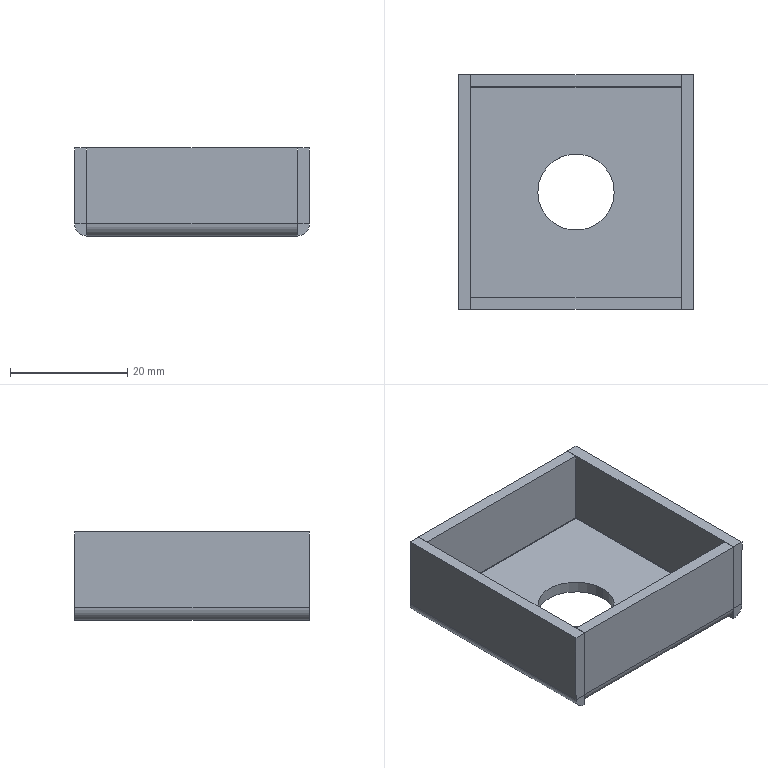Part | SolidWorks | features EdgeFlange 2, FlatPattern 1, ICE 1, SMBaseFlange 1, SheetMetal 1 | 1 solid | 44 faces | box 40 x 40 x 15 mm | volume 6733 mm3 | plane 34 | cylinder 10 | commonest cylinder face diameters 0.2 x4 4.2 x4 13 x2
STEP:
#1=CARTESIAN_POINT('',(-6.5,0.,0.));
#2=VERTEX_POINT('',#1);
#3=CARTESIAN_POINT('',(6.5,0.,0.));
#4=VERTEX_POINT('',#3);
#5=CARTESIAN_POINT('',(0.,0.,0.));
#6=DIRECTION('',(0.,0.,1.));
#7=DIRECTION('',(1.,0.,0.));
#8=AXIS2_PLACEMENT_3D('',#5,#6,#7);
#9=CIRCLE('',#8,6.5);
#10=EDGE_CURVE('',#2,#4,#9,.T.);
#11=ORIENTED_EDGE('',*,*,#10,.T.);
#12=CARTESIAN_POINT('',(6.5,0.,-2.));
#13=VERTEX_POINT('',#12);
#14=CARTESIAN_POINT('',(6.5,0.,8.));
#15=DIRECTION('',(0.,0.,-1.));
#16=VECTOR('',#15,1000.);
#17=LINE('',#14,#16);
#18=EDGE_CURVE('',#4,#13,#17,.T.);
#19=ORIENTED_EDGE('',*,*,#18,.T.);
#20=CARTESIAN_POINT('',(-6.5,0.,-2.));
#21=VERTEX_POINT('',#20);
#22=CARTESIAN_POINT('',(0.,0.,-2.));
#23=DIRECTION('',(0.,0.,-1.));
#24=DIRECTION('',(-1.,0.,0.));
#25=AXIS2_PLACEMENT_3D('',#22,#23,#24);
#26=CIRCLE('',#25,6.5);
#27=EDGE_CURVE('',#13,#21,#26,.T.);
#28=ORIENTED_EDGE('',*,*,#27,.T.);
#29=CARTESIAN_POINT('',(-6.5,0.,8.));
#30=DIRECTION('',(0.,0.,-1.));
#31=VECTOR('',#30,1000.);
#32=LINE('',#29,#31);
#33=EDGE_CURVE('',#2,#21,#32,.T.);
#34=ORIENTED_EDGE('',*,*,#33,.F.);
#35=EDGE_LOOP('',(#11,#19,#28,#34));
#36=FACE_OUTER_BOUND('',#35,.T.);
#37=CARTESIAN_POINT('',(0.,0.,8.));
#38=DIRECTION('',(0.,0.,-1.));
#39=DIRECTION('',(-1.,0.,0.));
#40=AXIS2_PLACEMENT_3D('',#37,#38,#39);
#41=CYLINDRICAL_SURFACE('',#40,6.5);
#42=ADVANCED_FACE('',(#36),#41,.F.);
#43=CARTESIAN_POINT('',(-17.9,-20.,-2.));
#44=VERTEX_POINT('',#43);
#45=CARTESIAN_POINT('',(-17.9,-17.9,-2.));
#46=VERTEX_POINT('',#45);
#47=CARTESIAN_POINT('',(-17.9,-20.,-2.));
#48=DIRECTION('',(0.,1.,0.));
#49=VECTOR('',#48,1000.);
#50=LINE('',#47,#49);
#51=EDGE_CURVE('',#44,#46,#50,.T.);
#52=ORIENTED_EDGE('',*,*,#51,.T.);
#53=CARTESIAN_POINT('',(-17.9,-19.998,0.));
#54=VERTEX_POINT('',#53);
#55=CARTESIAN_POINT('',(-17.9,-17.9,0.1));
#56=DIRECTION('',(-1.,0.,0.));
#57=DIRECTION('',(0.,0.,-1.));
#58=AXIS2_PLACEMENT_3D('',#55,#56,#57);
#59=CIRCLE('',#58,2.1);
#60=EDGE_CURVE('',#46,#54,#59,.T.);
#61=ORIENTED_EDGE('',*,*,#60,.T.);
#62=CARTESIAN_POINT('',(-17.9,-20.,0.));
#63=VERTEX_POINT('',#62);
#64=CARTESIAN_POINT('',(-17.9,-20.,0.));
#65=DIRECTION('',(0.,1.,0.));
#66=VECTOR('',#65,1000.);
#67=LINE('',#64,#66);
#68=EDGE_CURVE('',#63,#54,#67,.T.);
#69=ORIENTED_EDGE('',*,*,#68,.F.);
#70=CARTESIAN_POINT('',(-17.9,-20.,0.));
#71=DIRECTION('',(0.,0.,-1.));
#72=VECTOR('',#71,1000.);
#73=LINE('',#70,#72);
#74=EDGE_CURVE('',#63,#44,#73,.T.);
#75=ORIENTED_EDGE('',*,*,#74,.T.);
#76=EDGE_LOOP('',(#52,#61,#69,#75));
#77=FACE_OUTER_BOUND('',#76,.T.);
#78=CARTESIAN_POINT('',(-17.9,-17.9,0.));
#79=DIRECTION('',(1.,0.,0.));
#80=DIRECTION('',(0.,0.,-1.));
#81=AXIS2_PLACEMENT_3D('',#78,#79,#80);
#82=PLANE('',#81);
#83=ADVANCED_FACE('',(#77),#82,.T.);
#84=CARTESIAN_POINT('',(17.9,-20.,0.));
#85=VERTEX_POINT('',#84);
#86=CARTESIAN_POINT('',(17.9,-19.998,0.));
#87=VERTEX_POINT('',#86);
#88=CARTESIAN_POINT('',(17.9,-20.,0.));
#89=DIRECTION('',(0.,1.,0.));
#90=VECTOR('',#89,1000.);
#91=LINE('',#88,#90);
#92=EDGE_CURVE('',#85,#87,#91,.T.);
#93=ORIENTED_EDGE('',*,*,#92,.T.);
#94=CARTESIAN_POINT('',(17.9,-17.9,-2.));
#95=VERTEX_POINT('',#94);
#96=CARTESIAN_POINT('',(17.9,-17.9,0.1));
#97=DIRECTION('',(1.,0.,0.));
#98=DIRECTION('',(0.,0.,-1.));
#99=AXIS2_PLACEMENT_3D('',#96,#97,#98);
#100=CIRCLE('',#99,2.1);
#101=EDGE_CURVE('',#87,#95,#100,.T.);
#102=ORIENTED_EDGE('',*,*,#101,.T.);
#103=CARTESIAN_POINT('',(17.9,-20.,-2.));
#104=VERTEX_POINT('',#103);
#105=CARTESIAN_POINT('',(17.9,20.,-2.));
#106=DIRECTION('',(0.,1.,0.));
#107=VECTOR('',#106,1000.);
#108=LINE('',#105,#107);
#109=EDGE_CURVE('',#104,#95,#108,.T.);
#110=ORIENTED_EDGE('',*,*,#109,.F.);
#111=CARTESIAN_POINT('',(17.9,-20.,0.));
#112=DIRECTION('',(0.,0.,-1.));
#113=VECTOR('',#112,1000.);
#114=LINE('',#111,#113);
#115=EDGE_CURVE('',#85,#104,#114,.T.);
#116=ORIENTED_EDGE('',*,*,#115,.F.);
#117=EDGE_LOOP('',(#93,#102,#110,#116));
#118=FACE_OUTER_BOUND('',#117,.T.);
#119=CARTESIAN_POINT('',(17.9,-20.,0.));
#120=DIRECTION('',(-1.,0.,0.));
#121=DIRECTION('',(0.,-1.,0.));
#122=AXIS2_PLACEMENT_3D('',#119,#120,#121);
#123=PLANE('',#122);
#124=ADVANCED_FACE('',(#118),#123,.T.);
#125=CARTESIAN_POINT('',(-17.9,20.,0.));
#126=VERTEX_POINT('',#125);
#127=CARTESIAN_POINT('',(-17.9,19.998,0.));
#128=VERTEX_POINT('',#127);
#129=CARTESIAN_POINT('',(-17.9,20.,0.));
#130=DIRECTION('',(0.,-1.,0.));
#131=VECTOR('',#130,1000.);
#132=LINE('',#129,#131);
#133=EDGE_CURVE('',#126,#128,#132,.T.);
#134=ORIENTED_EDGE('',*,*,#133,.T.);
#135=CARTESIAN_POINT('',(-17.9,17.9,-2.));
#136=VERTEX_POINT('',#135);
#137=CARTESIAN_POINT('',(-17.9,17.9,0.1));
#138=DIRECTION('',(-1.,0.,0.));
#139=DIRECTION('',(0.,0.,1.));
#140=AXIS2_PLACEMENT_3D('',#137,#138,#139);
#141=CIRCLE('',#140,2.1);
#142=EDGE_CURVE('',#128,#136,#141,.T.);
#143=ORIENTED_EDGE('',*,*,#142,.T.);
#144=CARTESIAN_POINT('',(-17.9,20.,-2.));
#145=VERTEX_POINT('',#144);
#146=CARTESIAN_POINT('',(-17.9,-20.,-2.));
#147=DIRECTION('',(0.,-1.,0.));
#148=VECTOR('',#147,1000.);
#149=LINE('',#146,#148);
#150=EDGE_CURVE('',#145,#136,#149,.T.);
#151=ORIENTED_EDGE('',*,*,#150,.F.);
#152=CARTESIAN_POINT('',(-17.9,20.,0.));
#153=DIRECTION('',(0.,0.,-1.));
#154=VECTOR('',#153,1000.);
#155=LINE('',#152,#154);
#156=EDGE_CURVE('',#126,#145,#155,.T.);
#157=ORIENTED_EDGE('',*,*,#156,.F.);
#158=EDGE_LOOP('',(#134,#143,#151,#157));
#159=FACE_OUTER_BOUND('',#158,.T.);
#160=CARTESIAN_POINT('',(-17.9,20.,0.));
#161=DIRECTION('',(1.,0.,0.));
#162=DIRECTION('',(0.,0.,-1.));
#163=AXIS2_PLACEMENT_3D('',#160,#161,#162);
#164=PLANE('',#163);
#165=ADVANCED_FACE('',(#159),#164,.T.);
#166=CARTESIAN_POINT('',(17.9,20.,-2.));
#167=VERTEX_POINT('',#166);
#168=CARTESIAN_POINT('',(17.9,17.9,-2.));
#169=VERTEX_POINT('',#168);
#170=CARTESIAN_POINT('',(17.9,20.,-2.));
#171=DIRECTION('',(0.,-1.,0.));
#172=VECTOR('',#171,1000.);
#173=LINE('',#170,#172);
#174=EDGE_CURVE('',#167,#169,#173,.T.);
#175=ORIENTED_EDGE('',*,*,#174,.T.);
#176=CARTESIAN_POINT('',(17.9,19.998,0.));
#177=VERTEX_POINT('',#176);
#178=CARTESIAN_POINT('',(17.9,17.9,0.1));
#179=DIRECTION('',(1.,0.,0.));
#180=DIRECTION('',(0.,0.,1.));
#181=AXIS2_PLACEMENT_3D('',#178,#179,#180);
#182=CIRCLE('',#181,2.1);
#183=EDGE_CURVE('',#169,#177,#182,.T.);
#184=ORIENTED_EDGE('',*,*,#183,.T.);
#185=CARTESIAN_POINT('',(17.9,20.,0.));
#186=VERTEX_POINT('',#185);
#187=CARTESIAN_POINT('',(17.9,20.,0.));
#188=DIRECTION('',(0.,-1.,0.));
#189=VECTOR('',#188,1000.);
#190=LINE('',#187,#189);
#191=EDGE_CURVE('',#186,#177,#190,.T.);
#192=ORIENTED_EDGE('',*,*,#191,.F.);
#193=CARTESIAN_POINT('',(17.9,20.,0.));
#194=DIRECTION('',(0.,0.,-1.));
#195=VECTOR('',#194,1000.);
#196=LINE('',#193,#195);
#197=EDGE_CURVE('',#186,#167,#196,.T.);
#198=ORIENTED_EDGE('',*,*,#197,.T.);
#199=EDGE_LOOP('',(#175,#184,#192,#198));
#200=FACE_OUTER_BOUND('',#199,.T.);
#201=CARTESIAN_POINT('',(17.9,17.9,0.));
#202=DIRECTION('',(-1.,0.,0.));
#203=DIRECTION('',(0.,0.,1.));
#204=AXIS2_PLACEMENT_3D('',#201,#202,#203);
#205=PLANE('',#204);
#206=ADVANCED_FACE('',(#200),#205,.T.);
#207=CARTESIAN_POINT('',(0.,0.,-2.));
#208=DIRECTION('',(0.,0.,-1.));
#209=DIRECTION('',(-1.,0.,0.));
#210=AXIS2_PLACEMENT_3D('',#207,#208,#209);
#211=CIRCLE('',#210,6.5);
#212=EDGE_CURVE('',#21,#13,#211,.T.);
#213=ORIENTED_EDGE('',*,*,#212,.F.);
#214=ORIENTED_EDGE('',*,*,#27,.F.);
#215=EDGE_LOOP('',(#213,#214));
#216=FACE_BOUND('',#215,.T.);
#217=CARTESIAN_POINT('',(17.9,-17.9,-2.));
#218=DIRECTION('',(-1.,0.,0.));
#219=VECTOR('',#218,1000.);
#220=LINE('',#217,#219);
#221=EDGE_CURVE('',#95,#46,#220,.T.);
#222=ORIENTED_EDGE('',*,*,#221,.T.);
#223=CARTESIAN_POINT('',(-17.9,-20.,-2.));
#224=DIRECTION('',(0.,1.,0.));
#225=VECTOR('',#224,1000.);
#226=LINE('',#223,#225);
#227=EDGE_CURVE('',#46,#136,#226,.T.);
#228=ORIENTED_EDGE('',*,*,#227,.T.);
#229=CARTESIAN_POINT('',(-17.9,17.9,-2.));
#230=DIRECTION('',(1.,0.,0.));
#231=VECTOR('',#230,1000.);
#232=LINE('',#229,#231);
#233=EDGE_CURVE('',#136,#169,#232,.T.);
#234=ORIENTED_EDGE('',*,*,#233,.T.);
#235=CARTESIAN_POINT('',(17.9,20.,-2.));
#236=DIRECTION('',(0.,-1.,0.));
#237=VECTOR('',#236,1000.);
#238=LINE('',#235,#237);
#239=EDGE_CURVE('',#169,#95,#238,.T.);
#240=ORIENTED_EDGE('',*,*,#239,.T.);
#241=EDGE_LOOP('',(#222,#228,#234,#240));
#242=FACE_OUTER_BOUND('',#241,.T.);
#243=CARTESIAN_POINT('',(0.,0.,-2.));
#244=DIRECTION('',(0.,0.,1.));
#245=DIRECTION('',(1.,0.,0.));
#246=AXIS2_PLACEMENT_3D('',#243,#244,#245);
#247=PLANE('',#246);
#248=ADVANCED_FACE('',(#216,#242),#247,.F.);
#249=ORIENTED_EDGE('',*,*,#10,.F.);
#250=CARTESIAN_POINT('',(0.,0.,0.));
#251=DIRECTION('',(0.,0.,1.));
#252=DIRECTION('',(1.,0.,0.));
#253=AXIS2_PLACEMENT_3D('',#250,#251,#252);
#254=CIRCLE('',#253,6.5);
#255=EDGE_CURVE('',#4,#2,#254,.T.);
#256=ORIENTED_EDGE('',*,*,#255,.F.);
#257=EDGE_LOOP('',(#249,#256));
#258=FACE_BOUND('',#257,.T.);
#259=CARTESIAN_POINT('',(-17.9,-17.9,0.));
#260=VERTEX_POINT('',#259);
#261=CARTESIAN_POINT('',(-17.9,17.9,0.));
#262=VERTEX_POINT('',#261);
#263=CARTESIAN_POINT('',(-17.9,-20.,0.));
#264=DIRECTION('',(0.,1.,0.));
#265=VECTOR('',#264,1000.);
#266=LINE('',#263,#265);
#267=EDGE_CURVE('',#260,#262,#266,.T.);
#268=ORIENTED_EDGE('',*,*,#267,.F.);
#269=CARTESIAN_POINT('',(17.9,-17.9,0.));
#270=VERTEX_POINT('',#269);
#271=CARTESIAN_POINT('',(17.9,-17.9,0.));
#272=DIRECTION('',(-1.,0.,0.));
#273=VECTOR('',#272,1000.);
#274=LINE('',#271,#273);
#275=EDGE_CURVE('',#270,#260,#274,.T.);
#276=ORIENTED_EDGE('',*,*,#275,.F.);
#277=CARTESIAN_POINT('',(17.9,17.9,0.));
#278=VERTEX_POINT('',#277);
#279=CARTESIAN_POINT('',(17.9,20.,0.));
#280=DIRECTION('',(0.,-1.,0.));
#281=VECTOR('',#280,1000.);
#282=LINE('',#279,#281);
#283=EDGE_CURVE('',#278,#270,#282,.T.);
#284=ORIENTED_EDGE('',*,*,#283,.F.);
#285=CARTESIAN_POINT('',(-17.9,17.9,0.));
#286=DIRECTION('',(1.,0.,0.));
#287=VECTOR('',#286,1000.);
#288=LINE('',#285,#287);
#289=EDGE_CURVE('',#262,#278,#288,.T.);
#290=ORIENTED_EDGE('',*,*,#289,.F.);
#291=EDGE_LOOP('',(#268,#276,#284,#290));
#292=FACE_OUTER_BOUND('',#291,.T.);
#293=CARTESIAN_POINT('',(0.,0.,0.));
#294=DIRECTION('',(0.,0.,1.));
#295=DIRECTION('',(1.,0.,0.));
#296=AXIS2_PLACEMENT_3D('',#293,#294,#295);
#297=PLANE('',#296);
#298=ADVANCED_FACE('',(#258,#292),#297,.T.);
#299=ORIENTED_EDGE('',*,*,#18,.F.);
#300=ORIENTED_EDGE('',*,*,#255,.T.);
#301=ORIENTED_EDGE('',*,*,#33,.T.);
#302=ORIENTED_EDGE('',*,*,#212,.T.);
#303=EDGE_LOOP('',(#299,#300,#301,#302));
#304=FACE_OUTER_BOUND('',#303,.T.);
#305=CARTESIAN_POINT('',(0.,0.,8.));
#306=DIRECTION('',(0.,0.,-1.));
#307=DIRECTION('',(-1.,0.,0.));
#308=AXIS2_PLACEMENT_3D('',#305,#306,#307);
#309=CYLINDRICAL_SURFACE('',#308,6.5);
#310=ADVANCED_FACE('',(#304),#309,.F.);
#311=CARTESIAN_POINT('',(-18.,20.,0.1));
#312=VERTEX_POINT('',#311);
#313=CARTESIAN_POINT('',(-20.,20.,0.1));
#314=VERTEX_POINT('',#313);
#315=CARTESIAN_POINT('',(-20.,20.,0.1));
#316=DIRECTION('',(-1.,0.,0.));
#317=VECTOR('',#316,1000.);
#318=LINE('',#315,#317);
#319=EDGE_CURVE('',#312,#314,#318,.T.);
#320=ORIENTED_EDGE('',*,*,#319,.F.);
#321=CARTESIAN_POINT('',(-17.9,20.,0.1));
#322=DIRECTION('',(0.,1.,0.));
#323=DIRECTION('',(0.,0.,-1.));
#324=AXIS2_PLACEMENT_3D('',#321,#322,#323);
#325=CIRCLE('',#324,0.1);
#326=EDGE_CURVE('',#126,#312,#325,.T.);
#327=ORIENTED_EDGE('',*,*,#326,.F.);
#328=ORIENTED_EDGE('',*,*,#156,.T.);
#329=CARTESIAN_POINT('',(-17.9,20.,0.1));
#330=DIRECTION('',(0.,1.,0.));
#331=DIRECTION('',(0.,0.,-1.));
#332=AXIS2_PLACEMENT_3D('',#329,#330,#331);
#333=CIRCLE('',#332,2.1);
#334=EDGE_CURVE('',#145,#314,#333,.T.);
#335=ORIENTED_EDGE('',*,*,#334,.T.);
#336=EDGE_LOOP('',(#320,#327,#328,#335));
#337=FACE_OUTER_BOUND('',#336,.T.);
#338=CARTESIAN_POINT('',(-17.9,20.,0.1));
#339=DIRECTION('',(0.,1.,0.));
#340=DIRECTION('',(0.,0.,1.));
#341=AXIS2_PLACEMENT_3D('',#338,#339,#340);
#342=PLANE('',#341);
#343=ADVANCED_FACE('',(#337),#342,.T.);
#344=CARTESIAN_POINT('',(-18.,-20.,0.1));
#345=VERTEX_POINT('',#344);
#346=CARTESIAN_POINT('',(-17.9,-20.,0.1));
#347=DIRECTION('',(0.,-1.,0.));
#348=DIRECTION('',(0.,0.,-1.));
#349=AXIS2_PLACEMENT_3D('',#346,#347,#348);
#350=CIRCLE('',#349,0.1);
#351=EDGE_CURVE('',#345,#63,#350,.T.);
#352=ORIENTED_EDGE('',*,*,#351,.F.);
#353=CARTESIAN_POINT('',(-20.,-20.,0.1));
#354=VERTEX_POINT('',#353);
#355=CARTESIAN_POINT('',(-18.,-20.,0.1));
#356=DIRECTION('',(-1.,0.,0.));
#357=VECTOR('',#356,1000.);
#358=LINE('',#355,#357);
#359=EDGE_CURVE('',#345,#354,#358,.T.);
#360=ORIENTED_EDGE('',*,*,#359,.T.);
#361=CARTESIAN_POINT('',(-17.9,-20.,0.1));
#362=DIRECTION('',(0.,-1.,0.));
#363=DIRECTION('',(0.,0.,-1.));
#364=AXIS2_PLACEMENT_3D('',#361,#362,#363);
#365=CIRCLE('',#364,2.1);
#366=EDGE_CURVE('',#354,#44,#365,.T.);
#367=ORIENTED_EDGE('',*,*,#366,.T.);
#368=ORIENTED_EDGE('',*,*,#74,.F.);
#369=EDGE_LOOP('',(#352,#360,#367,#368));
#370=FACE_OUTER_BOUND('',#369,.T.);
#371=CARTESIAN_POINT('',(-17.9,-20.,0.1));
#372=DIRECTION('',(0.,1.,0.));
#373=DIRECTION('',(0.,0.,1.));
#374=AXIS2_PLACEMENT_3D('',#371,#372,#373);
#375=PLANE('',#374);
#376=ADVANCED_FACE('',(#370),#375,.F.);
#377=ORIENTED_EDGE('',*,*,#51,.F.);
#378=ORIENTED_EDGE('',*,*,#366,.F.);
#379=CARTESIAN_POINT('',(-20.,0.,0.1));
#380=DIRECTION('',(0.,-1.,0.));
#381=VECTOR('',#380,1000.);
#382=LINE('',#379,#381);
#383=EDGE_CURVE('',#314,#354,#382,.T.);
#384=ORIENTED_EDGE('',*,*,#383,.F.);
#385=ORIENTED_EDGE('',*,*,#334,.F.);
#386=ORIENTED_EDGE('',*,*,#150,.T.);
#387=ORIENTED_EDGE('',*,*,#227,.F.);
#388=EDGE_LOOP('',(#377,#378,#384,#385,#386,#387));
#389=FACE_OUTER_BOUND('',#388,.T.);
#390=CARTESIAN_POINT('',(-17.9,-20.,0.1));
#391=DIRECTION('',(0.,-1.,0.));
#392=DIRECTION('',(-1.,0.,0.));
#393=AXIS2_PLACEMENT_3D('',#390,#391,#392);
#394=CYLINDRICAL_SURFACE('',#393,2.1);
#395=ADVANCED_FACE('',(#389),#394,.T.);
#396=ORIENTED_EDGE('',*,*,#68,.T.);
#397=CARTESIAN_POINT('',(-17.9,-20.,0.));
#398=DIRECTION('',(0.,1.,0.));
#399=VECTOR('',#398,1000.);
#400=LINE('',#397,#399);
#401=EDGE_CURVE('',#54,#260,#400,.T.);
#402=ORIENTED_EDGE('',*,*,#401,.T.);
#403=ORIENTED_EDGE('',*,*,#267,.T.);
#404=CARTESIAN_POINT('',(-17.9,20.,0.));
#405=DIRECTION('',(0.,-1.,0.));
#406=VECTOR('',#405,1000.);
#407=LINE('',#404,#406);
#408=EDGE_CURVE('',#128,#262,#407,.T.);
#409=ORIENTED_EDGE('',*,*,#408,.F.);
#410=ORIENTED_EDGE('',*,*,#133,.F.);
#411=ORIENTED_EDGE('',*,*,#326,.T.);
#412=CARTESIAN_POINT('',(-18.,20.,0.1));
#413=DIRECTION('',(0.,-1.,0.));
#414=VECTOR('',#413,1000.);
#415=LINE('',#412,#414);
#416=EDGE_CURVE('',#312,#345,#415,.T.);
#417=ORIENTED_EDGE('',*,*,#416,.T.);
#418=ORIENTED_EDGE('',*,*,#351,.T.);
#419=EDGE_LOOP('',(#396,#402,#403,#409,#410,#411,#417,#418));
#420=FACE_OUTER_BOUND('',#419,.T.);
#421=CARTESIAN_POINT('',(-17.9,-20.,0.1));
#422=DIRECTION('',(0.,-1.,0.));
#423=DIRECTION('',(-1.,0.,0.));
#424=AXIS2_PLACEMENT_3D('',#421,#422,#423);
#425=CYLINDRICAL_SURFACE('',#424,0.1);
#426=ADVANCED_FACE('',(#420),#425,.F.);
#427=CARTESIAN_POINT('',(-20.,-20.,13.));
#428=VERTEX_POINT('',#427);
#429=CARTESIAN_POINT('',(-20.,-20.,0.));
#430=DIRECTION('',(0.,0.,-1.));
#431=VECTOR('',#430,1000.);
#432=LINE('',#429,#431);
#433=EDGE_CURVE('',#428,#354,#432,.T.);
#434=ORIENTED_EDGE('',*,*,#433,.T.);
#435=ORIENTED_EDGE('',*,*,#359,.F.);
#436=CARTESIAN_POINT('',(-18.,-20.,13.));
#437=VERTEX_POINT('',#436);
#438=CARTESIAN_POINT('',(-18.,-20.,0.));
#439=DIRECTION('',(0.,0.,-1.));
#440=VECTOR('',#439,1000.);
#441=LINE('',#438,#440);
#442=EDGE_CURVE('',#437,#345,#441,.T.);
#443=ORIENTED_EDGE('',*,*,#442,.F.);
#444=CARTESIAN_POINT('',(-20.,-20.,13.));
#445=DIRECTION('',(1.,0.,0.));
#446=VECTOR('',#445,1000.);
#447=LINE('',#444,#446);
#448=EDGE_CURVE('',#428,#437,#447,.T.);
#449=ORIENTED_EDGE('',*,*,#448,.F.);
#450=EDGE_LOOP('',(#434,#435,#443,#449));
#451=FACE_OUTER_BOUND('',#450,.T.);
#452=CARTESIAN_POINT('',(-20.,-20.,0.));
#453=DIRECTION('',(0.,-1.,0.));
#454=DIRECTION('',(1.,0.,0.));
#455=AXIS2_PLACEMENT_3D('',#452,#453,#454);
#456=PLANE('',#455);
#457=ADVANCED_FACE('',(#451),#456,.T.);
#458=CARTESIAN_POINT('',(-18.,20.,13.));
#459=VERTEX_POINT('',#458);
#460=CARTESIAN_POINT('',(-18.,20.,0.));
#461=DIRECTION('',(0.,0.,1.));
#462=VECTOR('',#461,1000.);
#463=LINE('',#460,#462);
#464=EDGE_CURVE('',#312,#459,#463,.T.);
#465=ORIENTED_EDGE('',*,*,#464,.F.);
#466=ORIENTED_EDGE('',*,*,#319,.T.);
#467=CARTESIAN_POINT('',(-20.,20.,13.));
#468=VERTEX_POINT('',#467);
#469=CARTESIAN_POINT('',(-20.,20.,13.));
#470=DIRECTION('',(0.,0.,1.));
#471=VECTOR('',#470,1000.);
#472=LINE('',#469,#471);
#473=EDGE_CURVE('',#314,#468,#472,.T.);
#474=ORIENTED_EDGE('',*,*,#473,.T.);
#475=CARTESIAN_POINT('',(-20.,20.,13.));
#476=DIRECTION('',(1.,0.,0.));
#477=VECTOR('',#476,1000.);
#478=LINE('',#475,#477);
#479=EDGE_CURVE('',#468,#459,#478,.T.);
#480=ORIENTED_EDGE('',*,*,#479,.T.);
#481=EDGE_LOOP('',(#465,#466,#474,#480));
#482=FACE_OUTER_BOUND('',#481,.T.);
#483=CARTESIAN_POINT('',(-20.,20.,13.));
#484=DIRECTION('',(0.,1.,0.));
#485=DIRECTION('',(-1.,0.,0.));
#486=AXIS2_PLACEMENT_3D('',#483,#484,#485);
#487=PLANE('',#486);
#488=ADVANCED_FACE('',(#482),#487,.T.);
#489=ORIENTED_EDGE('',*,*,#473,.F.);
#490=ORIENTED_EDGE('',*,*,#383,.T.);
#491=ORIENTED_EDGE('',*,*,#433,.F.);
#492=CARTESIAN_POINT('',(-20.,-20.,13.));
#493=DIRECTION('',(0.,-1.,0.));
#494=VECTOR('',#493,1000.);
#495=LINE('',#492,#494);
#496=EDGE_CURVE('',#468,#428,#495,.T.);
#497=ORIENTED_EDGE('',*,*,#496,.F.);
#498=EDGE_LOOP('',(#489,#490,#491,#497));
#499=FACE_OUTER_BOUND('',#498,.T.);
#500=CARTESIAN_POINT('',(-20.,0.,0.));
#501=DIRECTION('',(-1.,0.,0.));
#502=DIRECTION('',(0.,0.,1.));
#503=AXIS2_PLACEMENT_3D('',#500,#501,#502);
#504=PLANE('',#503);
#505=ADVANCED_FACE('',(#499),#504,.T.);
#506=ORIENTED_EDGE('',*,*,#416,.F.);
#507=ORIENTED_EDGE('',*,*,#464,.T.);
#508=CARTESIAN_POINT('',(-18.,0.,13.));
#509=DIRECTION('',(0.,-1.,0.));
#510=VECTOR('',#509,1000.);
#511=LINE('',#508,#510);
#512=EDGE_CURVE('',#459,#437,#511,.T.);
#513=ORIENTED_EDGE('',*,*,#512,.T.);
#514=ORIENTED_EDGE('',*,*,#442,.T.);
#515=EDGE_LOOP('',(#506,#507,#513,#514));
#516=FACE_OUTER_BOUND('',#515,.T.);
#517=CARTESIAN_POINT('',(-18.,0.,0.));
#518=DIRECTION('',(-1.,0.,0.));
#519=DIRECTION('',(0.,0.,1.));
#520=AXIS2_PLACEMENT_3D('',#517,#518,#519);
#521=PLANE('',#520);
#522=ADVANCED_FACE('',(#516),#521,.F.);
#523=ORIENTED_EDGE('',*,*,#512,.F.);
#524=ORIENTED_EDGE('',*,*,#479,.F.);
#525=ORIENTED_EDGE('',*,*,#496,.T.);
#526=ORIENTED_EDGE('',*,*,#448,.T.);
#527=EDGE_LOOP('',(#523,#524,#525,#526));
#528=FACE_OUTER_BOUND('',#527,.T.);
#529=CARTESIAN_POINT('',(-20.,-20.,13.));
#530=DIRECTION('',(0.,0.,1.));
#531=DIRECTION('',(1.,0.,0.));
#532=AXIS2_PLACEMENT_3D('',#529,#530,#531);
#533=PLANE('',#532);
#534=ADVANCED_FACE('',(#528),#533,.T.);
#535=CARTESIAN_POINT('',(18.,-20.,0.1));
#536=VERTEX_POINT('',#535);
#537=CARTESIAN_POINT('',(20.,-20.,0.1));
#538=VERTEX_POINT('',#537);
#539=CARTESIAN_POINT('',(20.,-20.,0.1));
#540=DIRECTION('',(1.,0.,0.));
#541=VECTOR('',#540,1000.);
#542=LINE('',#539,#541);
#543=EDGE_CURVE('',#536,#538,#542,.T.);
#544=ORIENTED_EDGE('',*,*,#543,.F.);
#545=CARTESIAN_POINT('',(17.9,-20.,0.1));
#546=DIRECTION('',(0.,-1.,0.));
#547=DIRECTION('',(0.,0.,1.));
#548=AXIS2_PLACEMENT_3D('',#545,#546,#547);
#549=CIRCLE('',#548,0.1);
#550=EDGE_CURVE('',#85,#536,#549,.T.);
#551=ORIENTED_EDGE('',*,*,#550,.F.);
#552=ORIENTED_EDGE('',*,*,#115,.T.);
#553=CARTESIAN_POINT('',(17.9,-20.,0.1));
#554=DIRECTION('',(0.,-1.,0.));
#555=DIRECTION('',(0.,0.,1.));
#556=AXIS2_PLACEMENT_3D('',#553,#554,#555);
#557=CIRCLE('',#556,2.1);
#558=EDGE_CURVE('',#104,#538,#557,.T.);
#559=ORIENTED_EDGE('',*,*,#558,.T.);
#560=EDGE_LOOP('',(#544,#551,#552,#559));
#561=FACE_OUTER_BOUND('',#560,.T.);
#562=CARTESIAN_POINT('',(17.9,-20.,0.1));
#563=DIRECTION('',(0.,-1.,0.));
#564=DIRECTION('',(0.,0.,-1.));
#565=AXIS2_PLACEMENT_3D('',#562,#563,#564);
#566=PLANE('',#565);
#567=ADVANCED_FACE('',(#561),#566,.T.);
#568=CARTESIAN_POINT('',(18.,20.,0.1));
#569=VERTEX_POINT('',#568);
#570=CARTESIAN_POINT('',(17.9,20.,0.1));
#571=DIRECTION('',(0.,1.,0.));
#572=DIRECTION('',(0.,0.,1.));
#573=AXIS2_PLACEMENT_3D('',#570,#571,#572);
#574=CIRCLE('',#573,0.1);
#575=EDGE_CURVE('',#569,#186,#574,.T.);
#576=ORIENTED_EDGE('',*,*,#575,.F.);
#577=CARTESIAN_POINT('',(20.,20.,0.1));
#578=VERTEX_POINT('',#577);
#579=CARTESIAN_POINT('',(18.,20.,0.1));
#580=DIRECTION('',(1.,0.,0.));
#581=VECTOR('',#580,1000.);
#582=LINE('',#579,#581);
#583=EDGE_CURVE('',#569,#578,#582,.T.);
#584=ORIENTED_EDGE('',*,*,#583,.T.);
#585=CARTESIAN_POINT('',(17.9,20.,0.1));
#586=DIRECTION('',(0.,1.,0.));
#587=DIRECTION('',(0.,0.,1.));
#588=AXIS2_PLACEMENT_3D('',#585,#586,#587);
#589=CIRCLE('',#588,2.1);
#590=EDGE_CURVE('',#578,#167,#589,.T.);
#591=ORIENTED_EDGE('',*,*,#590,.T.);
#592=ORIENTED_EDGE('',*,*,#197,.F.);
#593=EDGE_LOOP('',(#576,#584,#591,#592));
#594=FACE_OUTER_BOUND('',#593,.T.);
#595=CARTESIAN_POINT('',(17.9,20.,0.1));
#596=DIRECTION('',(0.,-1.,0.));
#597=DIRECTION('',(0.,0.,-1.));
#598=AXIS2_PLACEMENT_3D('',#595,#596,#597);
#599=PLANE('',#598);
#600=ADVANCED_FACE('',(#594),#599,.F.);
#601=ORIENTED_EDGE('',*,*,#174,.F.);
#602=ORIENTED_EDGE('',*,*,#590,.F.);
#603=CARTESIAN_POINT('',(20.,-20.,0.1));
#604=DIRECTION('',(0.,-1.,0.));
#605=VECTOR('',#604,1000.);
#606=LINE('',#603,#605);
#607=EDGE_CURVE('',#578,#538,#606,.T.);
#608=ORIENTED_EDGE('',*,*,#607,.T.);
#609=ORIENTED_EDGE('',*,*,#558,.F.);
#610=ORIENTED_EDGE('',*,*,#109,.T.);
#611=ORIENTED_EDGE('',*,*,#239,.F.);
#612=EDGE_LOOP('',(#601,#602,#608,#609,#610,#611));
#613=FACE_OUTER_BOUND('',#612,.T.);
#614=CARTESIAN_POINT('',(17.9,20.,0.1));
#615=DIRECTION('',(0.,1.,0.));
#616=DIRECTION('',(1.,0.,0.));
#617=AXIS2_PLACEMENT_3D('',#614,#615,#616);
#618=CYLINDRICAL_SURFACE('',#617,2.1);
#619=ADVANCED_FACE('',(#613),#618,.T.);
#620=ORIENTED_EDGE('',*,*,#191,.T.);
#621=CARTESIAN_POINT('',(17.9,20.,0.));
#622=DIRECTION('',(0.,-1.,0.));
#623=VECTOR('',#622,1000.);
#624=LINE('',#621,#623);
#625=EDGE_CURVE('',#177,#278,#624,.T.);
#626=ORIENTED_EDGE('',*,*,#625,.T.);
#627=ORIENTED_EDGE('',*,*,#283,.T.);
#628=CARTESIAN_POINT('',(17.9,-20.,0.));
#629=DIRECTION('',(0.,1.,0.));
#630=VECTOR('',#629,1000.);
#631=LINE('',#628,#630);
#632=EDGE_CURVE('',#87,#270,#631,.T.);
#633=ORIENTED_EDGE('',*,*,#632,.F.);
#634=ORIENTED_EDGE('',*,*,#92,.F.);
#635=ORIENTED_EDGE('',*,*,#550,.T.);
#636=CARTESIAN_POINT('',(18.,-20.,0.1));
#637=DIRECTION('',(0.,1.,0.));
#638=VECTOR('',#637,1000.);
#639=LINE('',#636,#638);
#640=EDGE_CURVE('',#536,#569,#639,.T.);
#641=ORIENTED_EDGE('',*,*,#640,.T.);
#642=ORIENTED_EDGE('',*,*,#575,.T.);
#643=EDGE_LOOP('',(#620,#626,#627,#633,#634,#635,#641,#642));
#644=FACE_OUTER_BOUND('',#643,.T.);
#645=CARTESIAN_POINT('',(17.9,20.,0.1));
#646=DIRECTION('',(0.,1.,0.));
#647=DIRECTION('',(1.,0.,0.));
#648=AXIS2_PLACEMENT_3D('',#645,#646,#647);
#649=CYLINDRICAL_SURFACE('',#648,0.1);
#650=ADVANCED_FACE('',(#644),#649,.F.);
#651=CARTESIAN_POINT('',(18.,-20.,13.));
#652=VERTEX_POINT('',#651);
#653=CARTESIAN_POINT('',(18.,-20.,0.));
#654=DIRECTION('',(0.,0.,1.));
#655=VECTOR('',#654,1000.);
#656=LINE('',#653,#655);
#657=EDGE_CURVE('',#536,#652,#656,.T.);
#658=ORIENTED_EDGE('',*,*,#657,.F.);
#659=ORIENTED_EDGE('',*,*,#543,.T.);
#660=CARTESIAN_POINT('',(20.,-20.,13.));
#661=VERTEX_POINT('',#660);
#662=CARTESIAN_POINT('',(20.,-20.,0.));
#663=DIRECTION('',(0.,0.,1.));
#664=VECTOR('',#663,1000.);
#665=LINE('',#662,#664);
#666=EDGE_CURVE('',#538,#661,#665,.T.);
#667=ORIENTED_EDGE('',*,*,#666,.T.);
#668=CARTESIAN_POINT('',(20.,-20.,13.));
#669=DIRECTION('',(-1.,0.,0.));
#670=VECTOR('',#669,1000.);
#671=LINE('',#668,#670);
#672=EDGE_CURVE('',#661,#652,#671,.T.);
#673=ORIENTED_EDGE('',*,*,#672,.T.);
#674=EDGE_LOOP('',(#658,#659,#667,#673));
#675=FACE_OUTER_BOUND('',#674,.T.);
#676=CARTESIAN_POINT('',(20.,-20.,0.));
#677=DIRECTION('',(0.,-1.,0.));
#678=DIRECTION('',(0.,0.,-1.));
#679=AXIS2_PLACEMENT_3D('',#676,#677,#678);
#680=PLANE('',#679);
#681=ADVANCED_FACE('',(#675),#680,.T.);
#682=CARTESIAN_POINT('',(20.,20.,13.));
#683=VERTEX_POINT('',#682);
#684=CARTESIAN_POINT('',(20.,20.,13.));
#685=DIRECTION('',(0.,0.,-1.));
#686=VECTOR('',#685,1000.);
#687=LINE('',#684,#686);
#688=EDGE_CURVE('',#683,#578,#687,.T.);
#689=ORIENTED_EDGE('',*,*,#688,.T.);
#690=ORIENTED_EDGE('',*,*,#583,.F.);
#691=CARTESIAN_POINT('',(18.,20.,13.));
#692=VERTEX_POINT('',#691);
#693=CARTESIAN_POINT('',(18.,20.,0.));
#694=DIRECTION('',(0.,0.,-1.));
#695=VECTOR('',#694,1000.);
#696=LINE('',#693,#695);
#697=EDGE_CURVE('',#692,#569,#696,.T.);
#698=ORIENTED_EDGE('',*,*,#697,.F.);
#699=CARTESIAN_POINT('',(20.,20.,13.));
#700=DIRECTION('',(-1.,0.,0.));
#701=VECTOR('',#700,1000.);
#702=LINE('',#699,#701);
#703=EDGE_CURVE('',#683,#692,#702,.T.);
#704=ORIENTED_EDGE('',*,*,#703,.F.);
#705=EDGE_LOOP('',(#689,#690,#698,#704));
#706=FACE_OUTER_BOUND('',#705,.T.);
#707=CARTESIAN_POINT('',(20.,20.,13.));
#708=DIRECTION('',(0.,1.,0.));
#709=DIRECTION('',(0.,0.,1.));
#710=AXIS2_PLACEMENT_3D('',#707,#708,#709);
#711=PLANE('',#710);
#712=ADVANCED_FACE('',(#706),#711,.T.);
#713=ORIENTED_EDGE('',*,*,#607,.F.);
#714=ORIENTED_EDGE('',*,*,#688,.F.);
#715=CARTESIAN_POINT('',(20.,-20.,13.));
#716=DIRECTION('',(0.,1.,0.));
#717=VECTOR('',#716,1000.);
#718=LINE('',#715,#717);
#719=EDGE_CURVE('',#661,#683,#718,.T.);
#720=ORIENTED_EDGE('',*,*,#719,.F.);
#721=ORIENTED_EDGE('',*,*,#666,.F.);
#722=EDGE_LOOP('',(#713,#714,#720,#721));
#723=FACE_OUTER_BOUND('',#722,.T.);
#724=CARTESIAN_POINT('',(20.,0.,0.));
#725=DIRECTION('',(-1.,0.,0.));
#726=DIRECTION('',(0.,0.,1.));
#727=AXIS2_PLACEMENT_3D('',#724,#725,#726);
#728=PLANE('',#727);
#729=ADVANCED_FACE('',(#723),#728,.F.);
#730=ORIENTED_EDGE('',*,*,#697,.T.);
#731=ORIENTED_EDGE('',*,*,#640,.F.);
#732=ORIENTED_EDGE('',*,*,#657,.T.);
#733=CARTESIAN_POINT('',(18.,0.,13.));
#734=DIRECTION('',(0.,1.,0.));
#735=VECTOR('',#734,1000.);
#736=LINE('',#733,#735);
#737=EDGE_CURVE('',#652,#692,#736,.T.);
#738=ORIENTED_EDGE('',*,*,#737,.T.);
#739=EDGE_LOOP('',(#730,#731,#732,#738));
#740=FACE_OUTER_BOUND('',#739,.T.);
#741=CARTESIAN_POINT('',(18.,0.,0.));
#742=DIRECTION('',(-1.,0.,0.));
#743=DIRECTION('',(0.,0.,1.));
#744=AXIS2_PLACEMENT_3D('',#741,#742,#743);
#745=PLANE('',#744);
#746=ADVANCED_FACE('',(#740),#745,.T.);
#747=ORIENTED_EDGE('',*,*,#737,.F.);
#748=ORIENTED_EDGE('',*,*,#672,.F.);
#749=ORIENTED_EDGE('',*,*,#719,.T.);
#750=ORIENTED_EDGE('',*,*,#703,.T.);
#751=EDGE_LOOP('',(#747,#748,#749,#750));
#752=FACE_OUTER_BOUND('',#751,.T.);
#753=CARTESIAN_POINT('',(20.,-20.,13.));
#754=DIRECTION('',(0.,0.,1.));
#755=DIRECTION('',(1.,0.,0.));
#756=AXIS2_PLACEMENT_3D('',#753,#754,#755);
#757=PLANE('',#756);
#758=ADVANCED_FACE('',(#752),#757,.T.);
#759=ORIENTED_EDGE('',*,*,#625,.F.);
#760=CARTESIAN_POINT('',(17.9,20.,0.1));
#761=VERTEX_POINT('',#760);
#762=CARTESIAN_POINT('',(17.9,17.9,0.1));
#763=DIRECTION('',(1.,0.,0.));
#764=DIRECTION('',(0.,0.,1.));
#765=AXIS2_PLACEMENT_3D('',#762,#763,#764);
#766=CIRCLE('',#765,2.1);
#767=EDGE_CURVE('',#177,#761,#766,.T.);
#768=ORIENTED_EDGE('',*,*,#767,.T.);
#769=CARTESIAN_POINT('',(17.9,18.,0.1));
#770=VERTEX_POINT('',#769);
#771=CARTESIAN_POINT('',(17.9,20.,0.1));
#772=DIRECTION('',(0.,1.,0.));
#773=VECTOR('',#772,1000.);
#774=LINE('',#771,#773);
#775=EDGE_CURVE('',#770,#761,#774,.T.);
#776=ORIENTED_EDGE('',*,*,#775,.F.);
#777=CARTESIAN_POINT('',(17.9,17.9,0.1));
#778=DIRECTION('',(1.,0.,0.));
#779=DIRECTION('',(0.,0.,1.));
#780=AXIS2_PLACEMENT_3D('',#777,#778,#779);
#781=CIRCLE('',#780,0.1);
#782=EDGE_CURVE('',#278,#770,#781,.T.);
#783=ORIENTED_EDGE('',*,*,#782,.F.);
#784=EDGE_LOOP('',(#759,#768,#776,#783));
#785=FACE_OUTER_BOUND('',#784,.T.);
#786=CARTESIAN_POINT('',(17.9,17.9,0.1));
#787=DIRECTION('',(1.,0.,0.));
#788=DIRECTION('',(0.,0.,-1.));
#789=AXIS2_PLACEMENT_3D('',#786,#787,#788);
#790=PLANE('',#789);
#791=ADVANCED_FACE('',(#785),#790,.T.);
#792=CARTESIAN_POINT('',(-17.9,20.,0.1));
#793=VERTEX_POINT('',#792);
#794=CARTESIAN_POINT('',(-17.9,17.9,0.1));
#795=DIRECTION('',(-1.,0.,0.));
#796=DIRECTION('',(0.,0.,1.));
#797=AXIS2_PLACEMENT_3D('',#794,#795,#796);
#798=CIRCLE('',#797,2.1);
#799=EDGE_CURVE('',#793,#128,#798,.T.);
#800=ORIENTED_EDGE('',*,*,#799,.T.);
#801=ORIENTED_EDGE('',*,*,#408,.T.);
#802=CARTESIAN_POINT('',(-17.9,18.,0.1));
#803=VERTEX_POINT('',#802);
#804=CARTESIAN_POINT('',(-17.9,17.9,0.1));
#805=DIRECTION('',(-1.,0.,0.));
#806=DIRECTION('',(0.,0.,1.));
#807=AXIS2_PLACEMENT_3D('',#804,#805,#806);
#808=CIRCLE('',#807,0.1);
#809=EDGE_CURVE('',#803,#262,#808,.T.);
#810=ORIENTED_EDGE('',*,*,#809,.F.);
#811=CARTESIAN_POINT('',(-17.9,18.,0.1));
#812=DIRECTION('',(0.,1.,0.));
#813=VECTOR('',#812,1000.);
#814=LINE('',#811,#813);
#815=EDGE_CURVE('',#803,#793,#814,.T.);
#816=ORIENTED_EDGE('',*,*,#815,.T.);
#817=EDGE_LOOP('',(#800,#801,#810,#816));
#818=FACE_OUTER_BOUND('',#817,.T.);
#819=CARTESIAN_POINT('',(-17.9,17.9,0.1));
#820=DIRECTION('',(1.,0.,0.));
#821=DIRECTION('',(0.,0.,-1.));
#822=AXIS2_PLACEMENT_3D('',#819,#820,#821);
#823=PLANE('',#822);
#824=ADVANCED_FACE('',(#818),#823,.F.);
#825=ORIENTED_EDGE('',*,*,#233,.F.);
#826=ORIENTED_EDGE('',*,*,#142,.F.);
#827=ORIENTED_EDGE('',*,*,#799,.F.);
#828=CARTESIAN_POINT('',(0.,20.,0.1));
#829=DIRECTION('',(-1.,0.,0.));
#830=VECTOR('',#829,1000.);
#831=LINE('',#828,#830);
#832=EDGE_CURVE('',#761,#793,#831,.T.);
#833=ORIENTED_EDGE('',*,*,#832,.F.);
#834=ORIENTED_EDGE('',*,*,#767,.F.);
#835=ORIENTED_EDGE('',*,*,#183,.F.);
#836=EDGE_LOOP('',(#825,#826,#827,#833,#834,#835));
#837=FACE_OUTER_BOUND('',#836,.T.);
#838=CARTESIAN_POINT('',(-17.9,17.9,0.1));
#839=DIRECTION('',(-1.,0.,0.));
#840=DIRECTION('',(0.,1.,0.));
#841=AXIS2_PLACEMENT_3D('',#838,#839,#840);
#842=CYLINDRICAL_SURFACE('',#841,2.1);
#843=ADVANCED_FACE('',(#837),#842,.T.);
#844=ORIENTED_EDGE('',*,*,#289,.T.);
#845=ORIENTED_EDGE('',*,*,#782,.T.);
#846=CARTESIAN_POINT('',(17.9,18.,0.1));
#847=DIRECTION('',(-1.,0.,0.));
#848=VECTOR('',#847,1000.);
#849=LINE('',#846,#848);
#850=EDGE_CURVE('',#770,#803,#849,.T.);
#851=ORIENTED_EDGE('',*,*,#850,.T.);
#852=ORIENTED_EDGE('',*,*,#809,.T.);
#853=EDGE_LOOP('',(#844,#845,#851,#852));
#854=FACE_OUTER_BOUND('',#853,.T.);
#855=CARTESIAN_POINT('',(-17.9,17.9,0.1));
#856=DIRECTION('',(-1.,0.,0.));
#857=DIRECTION('',(0.,1.,0.));
#858=AXIS2_PLACEMENT_3D('',#855,#856,#857);
#859=CYLINDRICAL_SURFACE('',#858,0.1);
#860=ADVANCED_FACE('',(#854),#859,.F.);
#861=CARTESIAN_POINT('',(-17.9,20.,13.));
#862=VERTEX_POINT('',#861);
#863=CARTESIAN_POINT('',(-17.9,20.,0.));
#864=DIRECTION('',(0.,0.,-1.));
#865=VECTOR('',#864,1000.);
#866=LINE('',#863,#865);
#867=EDGE_CURVE('',#862,#793,#866,.T.);
#868=ORIENTED_EDGE('',*,*,#867,.T.);
#869=ORIENTED_EDGE('',*,*,#815,.F.);
#870=CARTESIAN_POINT('',(-17.9,18.,13.));
#871=VERTEX_POINT('',#870);
#872=CARTESIAN_POINT('',(-17.9,18.,0.));
#873=DIRECTION('',(0.,0.,-1.));
#874=VECTOR('',#873,1000.);
#875=LINE('',#872,#874);
#876=EDGE_CURVE('',#871,#803,#875,.T.);
#877=ORIENTED_EDGE('',*,*,#876,.F.);
#878=CARTESIAN_POINT('',(-17.9,20.,13.));
#879=DIRECTION('',(0.,-1.,0.));
#880=VECTOR('',#879,1000.);
#881=LINE('',#878,#880);
#882=EDGE_CURVE('',#862,#871,#881,.T.);
#883=ORIENTED_EDGE('',*,*,#882,.F.);
#884=EDGE_LOOP('',(#868,#869,#877,#883));
#885=FACE_OUTER_BOUND('',#884,.T.);
#886=CARTESIAN_POINT('',(-17.9,20.,0.));
#887=DIRECTION('',(-1.,0.,0.));
#888=DIRECTION('',(0.,0.,1.));
#889=AXIS2_PLACEMENT_3D('',#886,#887,#888);
#890=PLANE('',#889);
#891=ADVANCED_FACE('',(#885),#890,.T.);
#892=CARTESIAN_POINT('',(17.9,18.,13.));
#893=VERTEX_POINT('',#892);
#894=CARTESIAN_POINT('',(17.9,18.,0.));
#895=DIRECTION('',(0.,0.,1.));
#896=VECTOR('',#895,1000.);
#897=LINE('',#894,#896);
#898=EDGE_CURVE('',#770,#893,#897,.T.);
#899=ORIENTED_EDGE('',*,*,#898,.F.);
#900=ORIENTED_EDGE('',*,*,#775,.T.);
#901=CARTESIAN_POINT('',(17.9,20.,13.));
#902=VERTEX_POINT('',#901);
#903=CARTESIAN_POINT('',(17.9,20.,13.));
#904=DIRECTION('',(0.,0.,1.));
#905=VECTOR('',#904,1000.);
#906=LINE('',#903,#905);
#907=EDGE_CURVE('',#761,#902,#906,.T.);
#908=ORIENTED_EDGE('',*,*,#907,.T.);
#909=CARTESIAN_POINT('',(17.9,20.,13.));
#910=DIRECTION('',(0.,-1.,0.));
#911=VECTOR('',#910,1000.);
#912=LINE('',#909,#911);
#913=EDGE_CURVE('',#902,#893,#912,.T.);
#914=ORIENTED_EDGE('',*,*,#913,.T.);
#915=EDGE_LOOP('',(#899,#900,#908,#914));
#916=FACE_OUTER_BOUND('',#915,.T.);
#917=CARTESIAN_POINT('',(17.9,20.,13.));
#918=DIRECTION('',(1.,0.,0.));
#919=DIRECTION('',(0.,0.,-1.));
#920=AXIS2_PLACEMENT_3D('',#917,#918,#919);
#921=PLANE('',#920);
#922=ADVANCED_FACE('',(#916),#921,.T.);
#923=ORIENTED_EDGE('',*,*,#907,.F.);
#924=ORIENTED_EDGE('',*,*,#832,.T.);
#925=ORIENTED_EDGE('',*,*,#867,.F.);
#926=CARTESIAN_POINT('',(-17.9,20.,13.));
#927=DIRECTION('',(-1.,0.,0.));
#928=VECTOR('',#927,1000.);
#929=LINE('',#926,#928);
#930=EDGE_CURVE('',#902,#862,#929,.T.);
#931=ORIENTED_EDGE('',*,*,#930,.F.);
#932=EDGE_LOOP('',(#923,#924,#925,#931));
#933=FACE_OUTER_BOUND('',#932,.T.);
#934=CARTESIAN_POINT('',(0.,20.,0.));
#935=DIRECTION('',(0.,1.,0.));
#936=DIRECTION('',(0.,0.,1.));
#937=AXIS2_PLACEMENT_3D('',#934,#935,#936);
#938=PLANE('',#937);
#939=ADVANCED_FACE('',(#933),#938,.T.);
#940=ORIENTED_EDGE('',*,*,#850,.F.);
#941=ORIENTED_EDGE('',*,*,#898,.T.);
#942=CARTESIAN_POINT('',(0.,18.,13.));
#943=DIRECTION('',(-1.,0.,0.));
#944=VECTOR('',#943,1000.);
#945=LINE('',#942,#944);
#946=EDGE_CURVE('',#893,#871,#945,.T.);
#947=ORIENTED_EDGE('',*,*,#946,.T.);
#948=ORIENTED_EDGE('',*,*,#876,.T.);
#949=EDGE_LOOP('',(#940,#941,#947,#948));
#950=FACE_OUTER_BOUND('',#949,.T.);
#951=CARTESIAN_POINT('',(0.,18.,0.));
#952=DIRECTION('',(0.,1.,0.));
#953=DIRECTION('',(0.,0.,1.));
#954=AXIS2_PLACEMENT_3D('',#951,#952,#953);
#955=PLANE('',#954);
#956=ADVANCED_FACE('',(#950),#955,.F.);
#957=ORIENTED_EDGE('',*,*,#946,.F.);
#958=ORIENTED_EDGE('',*,*,#913,.F.);
#959=ORIENTED_EDGE('',*,*,#930,.T.);
#960=ORIENTED_EDGE('',*,*,#882,.T.);
#961=EDGE_LOOP('',(#957,#958,#959,#960));
#962=FACE_OUTER_BOUND('',#961,.T.);
#963=CARTESIAN_POINT('',(-17.9,20.,13.));
#964=DIRECTION('',(0.,0.,1.));
#965=DIRECTION('',(0.,-1.,0.));
#966=AXIS2_PLACEMENT_3D('',#963,#964,#965);
#967=PLANE('',#966);
#968=ADVANCED_FACE('',(#962),#967,.T.);
#969=ORIENTED_EDGE('',*,*,#401,.F.);
#970=CARTESIAN_POINT('',(-17.9,-20.,0.1));
#971=VERTEX_POINT('',#970);
#972=CARTESIAN_POINT('',(-17.9,-17.9,0.1));
#973=DIRECTION('',(-1.,0.,0.));
#974=DIRECTION('',(0.,0.,-1.));
#975=AXIS2_PLACEMENT_3D('',#972,#973,#974);
#976=CIRCLE('',#975,2.1);
#977=EDGE_CURVE('',#54,#971,#976,.T.);
#978=ORIENTED_EDGE('',*,*,#977,.T.);
#979=CARTESIAN_POINT('',(-17.9,-18.,0.1));
#980=VERTEX_POINT('',#979);
#981=CARTESIAN_POINT('',(-17.9,-20.,0.1));
#982=DIRECTION('',(0.,-1.,0.));
#983=VECTOR('',#982,1000.);
#984=LINE('',#981,#983);
#985=EDGE_CURVE('',#980,#971,#984,.T.);
#986=ORIENTED_EDGE('',*,*,#985,.F.);
#987=CARTESIAN_POINT('',(-17.9,-17.9,0.1));
#988=DIRECTION('',(-1.,0.,0.));
#989=DIRECTION('',(0.,0.,-1.));
#990=AXIS2_PLACEMENT_3D('',#987,#988,#989);
#991=CIRCLE('',#990,0.1);
#992=EDGE_CURVE('',#260,#980,#991,.T.);
#993=ORIENTED_EDGE('',*,*,#992,.F.);
#994=EDGE_LOOP('',(#969,#978,#986,#993));
#995=FACE_OUTER_BOUND('',#994,.T.);
#996=CARTESIAN_POINT('',(-17.9,-17.9,0.1));
#997=DIRECTION('',(-1.,0.,0.));
#998=DIRECTION('',(0.,0.,1.));
#999=AXIS2_PLACEMENT_3D('',#996,#997,#998);
#1000=PLANE('',#999);
#1001=ADVANCED_FACE('',(#995),#1000,.T.);
#1002=CARTESIAN_POINT('',(17.9,-20.,0.1));
#1003=VERTEX_POINT('',#1002);
#1004=CARTESIAN_POINT('',(17.9,-17.9,0.1));
#1005=DIRECTION('',(1.,0.,0.));
#1006=DIRECTION('',(0.,0.,-1.));
#1007=AXIS2_PLACEMENT_3D('',#1004,#1005,#1006);
#1008=CIRCLE('',#1007,2.1);
#1009=EDGE_CURVE('',#1003,#87,#1008,.T.);
#1010=ORIENTED_EDGE('',*,*,#1009,.T.);
#1011=ORIENTED_EDGE('',*,*,#632,.T.);
#1012=CARTESIAN_POINT('',(17.9,-18.,0.1));
#1013=VERTEX_POINT('',#1012);
#1014=CARTESIAN_POINT('',(17.9,-17.9,0.1));
#1015=DIRECTION('',(1.,0.,0.));
#1016=DIRECTION('',(0.,0.,-1.));
#1017=AXIS2_PLACEMENT_3D('',#1014,#1015,#1016);
#1018=CIRCLE('',#1017,0.1);
#1019=EDGE_CURVE('',#1013,#270,#1018,.T.);
#1020=ORIENTED_EDGE('',*,*,#1019,.F.);
#1021=CARTESIAN_POINT('',(17.9,-18.,0.1));
#1022=DIRECTION('',(0.,-1.,0.));
#1023=VECTOR('',#1022,1000.);
#1024=LINE('',#1021,#1023);
#1025=EDGE_CURVE('',#1013,#1003,#1024,.T.);
#1026=ORIENTED_EDGE('',*,*,#1025,.T.);
#1027=EDGE_LOOP('',(#1010,#1011,#1020,#1026));
#1028=FACE_OUTER_BOUND('',#1027,.T.);
#1029=CARTESIAN_POINT('',(17.9,-17.9,0.1));
#1030=DIRECTION('',(-1.,0.,0.));
#1031=DIRECTION('',(0.,0.,1.));
#1032=AXIS2_PLACEMENT_3D('',#1029,#1030,#1031);
#1033=PLANE('',#1032);
#1034=ADVANCED_FACE('',(#1028),#1033,.F.);
#1035=ORIENTED_EDGE('',*,*,#221,.F.);
#1036=ORIENTED_EDGE('',*,*,#101,.F.);
#1037=ORIENTED_EDGE('',*,*,#1009,.F.);
#1038=CARTESIAN_POINT('',(-17.9,-20.,0.1));
#1039=DIRECTION('',(-1.,0.,0.));
#1040=VECTOR('',#1039,1000.);
#1041=LINE('',#1038,#1040);
#1042=EDGE_CURVE('',#1003,#971,#1041,.T.);
#1043=ORIENTED_EDGE('',*,*,#1042,.T.);
#1044=ORIENTED_EDGE('',*,*,#977,.F.);
#1045=ORIENTED_EDGE('',*,*,#60,.F.);
#1046=EDGE_LOOP('',(#1035,#1036,#1037,#1043,#1044,#1045));
#1047=FACE_OUTER_BOUND('',#1046,.T.);
#1048=CARTESIAN_POINT('',(17.9,-17.9,0.1));
#1049=DIRECTION('',(1.,0.,0.));
#1050=DIRECTION('',(0.,-1.,0.));
#1051=AXIS2_PLACEMENT_3D('',#1048,#1049,#1050);
#1052=CYLINDRICAL_SURFACE('',#1051,2.1);
#1053=ADVANCED_FACE('',(#1047),#1052,.T.);
#1054=ORIENTED_EDGE('',*,*,#275,.T.);
#1055=ORIENTED_EDGE('',*,*,#992,.T.);
#1056=CARTESIAN_POINT('',(-17.9,-18.,0.1));
#1057=DIRECTION('',(1.,0.,0.));
#1058=VECTOR('',#1057,1000.);
#1059=LINE('',#1056,#1058);
#1060=EDGE_CURVE('',#980,#1013,#1059,.T.);
#1061=ORIENTED_EDGE('',*,*,#1060,.T.);
#1062=ORIENTED_EDGE('',*,*,#1019,.T.);
#1063=EDGE_LOOP('',(#1054,#1055,#1061,#1062));
#1064=FACE_OUTER_BOUND('',#1063,.T.);
#1065=CARTESIAN_POINT('',(17.9,-17.9,0.1));
#1066=DIRECTION('',(1.,0.,0.));
#1067=DIRECTION('',(0.,-1.,0.));
#1068=AXIS2_PLACEMENT_3D('',#1065,#1066,#1067);
#1069=CYLINDRICAL_SURFACE('',#1068,0.1);
#1070=ADVANCED_FACE('',(#1064),#1069,.F.);
#1071=CARTESIAN_POINT('',(-17.9,-18.,13.));
#1072=VERTEX_POINT('',#1071);
#1073=CARTESIAN_POINT('',(-17.9,-18.,0.));
#1074=DIRECTION('',(0.,0.,1.));
#1075=VECTOR('',#1074,1000.);
#1076=LINE('',#1073,#1075);
#1077=EDGE_CURVE('',#980,#1072,#1076,.T.);
#1078=ORIENTED_EDGE('',*,*,#1077,.F.);
#1079=ORIENTED_EDGE('',*,*,#985,.T.);
#1080=CARTESIAN_POINT('',(-17.9,-20.,13.));
#1081=VERTEX_POINT('',#1080);
#1082=CARTESIAN_POINT('',(-17.9,-20.,0.));
#1083=DIRECTION('',(0.,0.,1.));
#1084=VECTOR('',#1083,1000.);
#1085=LINE('',#1082,#1084);
#1086=EDGE_CURVE('',#971,#1081,#1085,.T.);
#1087=ORIENTED_EDGE('',*,*,#1086,.T.);
#1088=CARTESIAN_POINT('',(-17.9,-20.,13.));
#1089=DIRECTION('',(0.,1.,0.));
#1090=VECTOR('',#1089,1000.);
#1091=LINE('',#1088,#1090);
#1092=EDGE_CURVE('',#1081,#1072,#1091,.T.);
#1093=ORIENTED_EDGE('',*,*,#1092,.T.);
#1094=EDGE_LOOP('',(#1078,#1079,#1087,#1093));
#1095=FACE_OUTER_BOUND('',#1094,.T.);
#1096=CARTESIAN_POINT('',(-17.9,-20.,0.));
#1097=DIRECTION('',(-1.,0.,0.));
#1098=DIRECTION('',(0.,-1.,0.));
#1099=AXIS2_PLACEMENT_3D('',#1096,#1097,#1098);
#1100=PLANE('',#1099);
#1101=ADVANCED_FACE('',(#1095),#1100,.T.);
#1102=CARTESIAN_POINT('',(17.9,-20.,13.));
#1103=VERTEX_POINT('',#1102);
#1104=CARTESIAN_POINT('',(17.9,-20.,13.));
#1105=DIRECTION('',(0.,0.,-1.));
#1106=VECTOR('',#1105,1000.);
#1107=LINE('',#1104,#1106);
#1108=EDGE_CURVE('',#1103,#1003,#1107,.T.);
#1109=ORIENTED_EDGE('',*,*,#1108,.T.);
#1110=ORIENTED_EDGE('',*,*,#1025,.F.);
#1111=CARTESIAN_POINT('',(17.9,-18.,13.));
#1112=VERTEX_POINT('',#1111);
#1113=CARTESIAN_POINT('',(17.9,-18.,0.));
#1114=DIRECTION('',(0.,0.,-1.));
#1115=VECTOR('',#1114,1000.);
#1116=LINE('',#1113,#1115);
#1117=EDGE_CURVE('',#1112,#1013,#1116,.T.);
#1118=ORIENTED_EDGE('',*,*,#1117,.F.);
#1119=CARTESIAN_POINT('',(17.9,-20.,13.));
#1120=DIRECTION('',(0.,1.,0.));
#1121=VECTOR('',#1120,1000.);
#1122=LINE('',#1119,#1121);
#1123=EDGE_CURVE('',#1103,#1112,#1122,.T.);
#1124=ORIENTED_EDGE('',*,*,#1123,.F.);
#1125=EDGE_LOOP('',(#1109,#1110,#1118,#1124));
#1126=FACE_OUTER_BOUND('',#1125,.T.);
#1127=CARTESIAN_POINT('',(17.9,-20.,13.));
#1128=DIRECTION('',(1.,0.,0.));
#1129=DIRECTION('',(0.,1.,0.));
#1130=AXIS2_PLACEMENT_3D('',#1127,#1128,#1129);
#1131=PLANE('',#1130);
#1132=ADVANCED_FACE('',(#1126),#1131,.T.);
#1133=ORIENTED_EDGE('',*,*,#1042,.F.);
#1134=ORIENTED_EDGE('',*,*,#1108,.F.);
#1135=CARTESIAN_POINT('',(-17.9,-20.,13.));
#1136=DIRECTION('',(1.,0.,0.));
#1137=VECTOR('',#1136,1000.);
#1138=LINE('',#1135,#1137);
#1139=EDGE_CURVE('',#1081,#1103,#1138,.T.);
#1140=ORIENTED_EDGE('',*,*,#1139,.F.);
#1141=ORIENTED_EDGE('',*,*,#1086,.F.);
#1142=EDGE_LOOP('',(#1133,#1134,#1140,#1141));
#1143=FACE_OUTER_BOUND('',#1142,.T.);
#1144=CARTESIAN_POINT('',(0.,-20.,0.));
#1145=DIRECTION('',(0.,1.,0.));
#1146=DIRECTION('',(0.,0.,1.));
#1147=AXIS2_PLACEMENT_3D('',#1144,#1145,#1146);
#1148=PLANE('',#1147);
#1149=ADVANCED_FACE('',(#1143),#1148,.F.);
#1150=ORIENTED_EDGE('',*,*,#1117,.T.);
#1151=ORIENTED_EDGE('',*,*,#1060,.F.);
#1152=ORIENTED_EDGE('',*,*,#1077,.T.);
#1153=CARTESIAN_POINT('',(0.,-18.,13.));
#1154=DIRECTION('',(1.,0.,0.));
#1155=VECTOR('',#1154,1000.);
#1156=LINE('',#1153,#1155);
#1157=EDGE_CURVE('',#1072,#1112,#1156,.T.);
#1158=ORIENTED_EDGE('',*,*,#1157,.T.);
#1159=EDGE_LOOP('',(#1150,#1151,#1152,#1158));
#1160=FACE_OUTER_BOUND('',#1159,.T.);
#1161=CARTESIAN_POINT('',(0.,-18.,0.));
#1162=DIRECTION('',(0.,1.,0.));
#1163=DIRECTION('',(0.,0.,1.));
#1164=AXIS2_PLACEMENT_3D('',#1161,#1162,#1163);
#1165=PLANE('',#1164);
#1166=ADVANCED_FACE('',(#1160),#1165,.T.);
#1167=ORIENTED_EDGE('',*,*,#1157,.F.);
#1168=ORIENTED_EDGE('',*,*,#1092,.F.);
#1169=ORIENTED_EDGE('',*,*,#1139,.T.);
#1170=ORIENTED_EDGE('',*,*,#1123,.T.);
#1171=EDGE_LOOP('',(#1167,#1168,#1169,#1170));
#1172=FACE_OUTER_BOUND('',#1171,.T.);
#1173=CARTESIAN_POINT('',(-17.9,-20.,13.));
#1174=DIRECTION('',(0.,0.,1.));
#1175=DIRECTION('',(0.,-1.,0.));
#1176=AXIS2_PLACEMENT_3D('',#1173,#1174,#1175);
#1177=PLANE('',#1176);
#1178=ADVANCED_FACE('',(#1172),#1177,.T.);
#1179=CLOSED_SHELL('',(#42,#83,#124,#165,#206,#248,#298,#310,#343,#376,#395,#426,#457,#488,#505,#522,#534,#567,#600,#619,#650,#681,#712,#729,#746,#758,#791,#824,#843,#860,#891,#922,#939,#956,#968,#1001,#1034,#1053,#1070,#1101,#1132,#1149,#1166,#1178));
#1180=MANIFOLD_SOLID_BREP('',#1179);
#1181=CARTESIAN_POINT('',(0.,0.,0.));
#1182=DIRECTION('',(0.,0.,1.));
#1183=DIRECTION('',(1.,0.,0.));
#1184=AXIS2_PLACEMENT_3D('',#1181,#1182,#1183);
#1185=(LENGTH_UNIT()NAMED_UNIT(*)SI_UNIT(.MILLI.,.METRE.));
#1186=UNCERTAINTY_MEASURE_WITH_UNIT(LENGTH_MEASURE(0.00001),#1185,'','');
#1187=(NAMED_UNIT(*)PLANE_ANGLE_UNIT()SI_UNIT($,.RADIAN.));
#1188=(NAMED_UNIT(*)SI_UNIT($,.STERADIAN.)SOLID_ANGLE_UNIT());
#1189=(GEOMETRIC_REPRESENTATION_CONTEXT(3)GLOBAL_UNCERTAINTY_ASSIGNED_CONTEXT((#1186))GLOBAL_UNIT_ASSIGNED_CONTEXT((#1185,#1187,#1188))REPRESENTATION_CONTEXT('',''));
#1190=ADVANCED_BREP_SHAPE_REPRESENTATION('',(#1180,#1184),#1189);